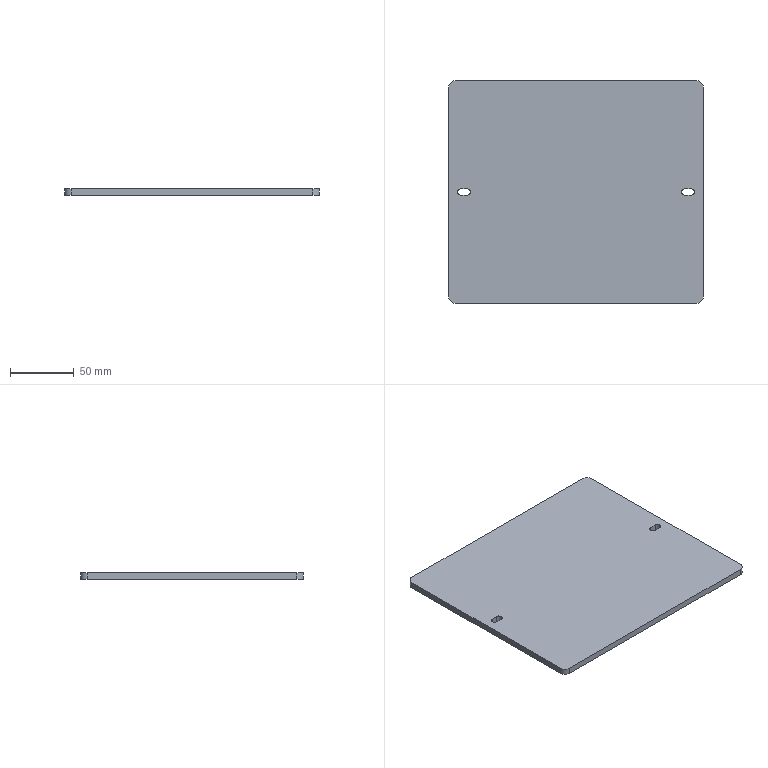Part | STEP file | ND25021-01-JDKM-01-SL | 1 solid | 20 faces | box 200 x 175 x 5 mm | volume 174446 mm3 | cylinder 10 | plane 10 | commonest cylinder face diameters 5 x6 10 x4